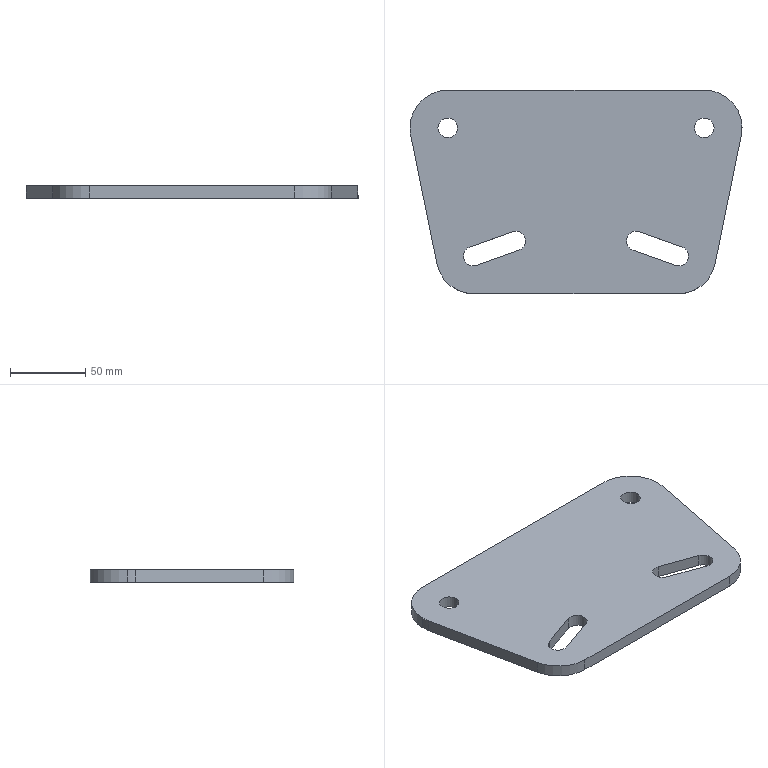Part | SolidWorks | features Extrusion 1 | 1 solid | 25 faces | box 220 x 135 x 8 mm | volume 204896 mm3 | cylinder 15 | plane 10 | commonest cylinder face diameters 13 x10 50 x5
STEP:
#1=CARTESIAN_POINT('',(163.5,-25.,8.));
#2=VERTEX_POINT('',#1);
#3=CARTESIAN_POINT('',(176.5,-25.,8.));
#4=VERTEX_POINT('',#3);
#5=CARTESIAN_POINT('',(170.,-25.,8.));
#6=DIRECTION('',(0.,0.,1.));
#7=DIRECTION('',(1.,0.,0.));
#8=AXIS2_PLACEMENT_3D('',#5,#6,#7);
#9=CIRCLE('',#8,6.5);
#10=EDGE_CURVE('',#2,#4,#9,.T.);
#11=ORIENTED_EDGE('',*,*,#10,.T.);
#12=CARTESIAN_POINT('',(176.5,-25.,0.));
#13=VERTEX_POINT('',#12);
#14=CARTESIAN_POINT('',(176.5,-25.,8.));
#15=DIRECTION('',(0.,0.,-1.));
#16=VECTOR('',#15,1000.);
#17=LINE('',#14,#16);
#18=EDGE_CURVE('',#4,#13,#17,.T.);
#19=ORIENTED_EDGE('',*,*,#18,.T.);
#20=CARTESIAN_POINT('',(163.5,-25.,0.));
#21=VERTEX_POINT('',#20);
#22=CARTESIAN_POINT('',(170.,-25.,0.));
#23=DIRECTION('',(0.,0.,1.));
#24=DIRECTION('',(1.,0.,0.));
#25=AXIS2_PLACEMENT_3D('',#22,#23,#24);
#26=CIRCLE('',#25,6.5);
#27=EDGE_CURVE('',#21,#13,#26,.T.);
#28=ORIENTED_EDGE('',*,*,#27,.F.);
#29=CARTESIAN_POINT('',(163.5,-25.,8.));
#30=DIRECTION('',(0.,0.,-1.));
#31=VECTOR('',#30,1000.);
#32=LINE('',#29,#31);
#33=EDGE_CURVE('',#2,#21,#32,.T.);
#34=ORIENTED_EDGE('',*,*,#33,.F.);
#35=EDGE_LOOP('',(#11,#19,#28,#34));
#36=FACE_OUTER_BOUND('',#35,.T.);
#37=CARTESIAN_POINT('',(170.,-25.,8.));
#38=DIRECTION('',(0.,0.,-1.));
#39=DIRECTION('',(-1.,0.,0.));
#40=AXIS2_PLACEMENT_3D('',#37,#38,#39);
#41=CYLINDRICAL_SURFACE('',#40,6.5);
#42=ADVANCED_FACE('',(#36),#41,.F.);
#43=CARTESIAN_POINT('',(14.814,-103.879,8.));
#44=VERTEX_POINT('',#43);
#45=CARTESIAN_POINT('',(10.5,-110.,8.));
#46=VERTEX_POINT('',#45);
#47=CARTESIAN_POINT('',(17.,-110.,8.));
#48=DIRECTION('',(0.,0.,1.));
#49=DIRECTION('',(1.,0.,0.));
#50=AXIS2_PLACEMENT_3D('',#47,#48,#49);
#51=CIRCLE('',#50,6.5);
#52=EDGE_CURVE('',#44,#46,#51,.T.);
#53=ORIENTED_EDGE('',*,*,#52,.T.);
#54=CARTESIAN_POINT('',(10.5,-110.,0.));
#55=VERTEX_POINT('',#54);
#56=CARTESIAN_POINT('',(10.5,-110.,8.));
#57=DIRECTION('',(0.,0.,-1.));
#58=VECTOR('',#57,1000.);
#59=LINE('',#56,#58);
#60=EDGE_CURVE('',#46,#55,#59,.T.);
#61=ORIENTED_EDGE('',*,*,#60,.T.);
#62=CARTESIAN_POINT('',(14.814,-103.879,0.));
#63=VERTEX_POINT('',#62);
#64=CARTESIAN_POINT('',(17.,-110.,0.));
#65=DIRECTION('',(0.,0.,1.));
#66=DIRECTION('',(1.,0.,0.));
#67=AXIS2_PLACEMENT_3D('',#64,#65,#66);
#68=CIRCLE('',#67,6.5);
#69=EDGE_CURVE('',#63,#55,#68,.T.);
#70=ORIENTED_EDGE('',*,*,#69,.F.);
#71=CARTESIAN_POINT('',(14.814,-103.879,8.));
#72=DIRECTION('',(0.,0.,-1.));
#73=VECTOR('',#72,1000.);
#74=LINE('',#71,#73);
#75=EDGE_CURVE('',#44,#63,#74,.T.);
#76=ORIENTED_EDGE('',*,*,#75,.F.);
#77=EDGE_LOOP('',(#53,#61,#70,#76));
#78=FACE_OUTER_BOUND('',#77,.T.);
#79=CARTESIAN_POINT('',(17.,-110.,8.));
#80=DIRECTION('',(0.,0.,-1.));
#81=DIRECTION('',(-1.,0.,0.));
#82=AXIS2_PLACEMENT_3D('',#79,#80,#81);
#83=CYLINDRICAL_SURFACE('',#82,6.5);
#84=ADVANCED_FACE('',(#78),#83,.F.);
#85=CARTESIAN_POINT('',(127.186,-93.879,8.));
#86=VERTEX_POINT('',#85);
#87=CARTESIAN_POINT('',(118.5,-100.,8.));
#88=VERTEX_POINT('',#87);
#89=CARTESIAN_POINT('',(125.,-100.,8.));
#90=DIRECTION('',(0.,0.,1.));
#91=DIRECTION('',(1.,0.,0.));
#92=AXIS2_PLACEMENT_3D('',#89,#90,#91);
#93=CIRCLE('',#92,6.5);
#94=EDGE_CURVE('',#86,#88,#93,.T.);
#95=ORIENTED_EDGE('',*,*,#94,.T.);
#96=CARTESIAN_POINT('',(118.5,-100.,0.));
#97=VERTEX_POINT('',#96);
#98=CARTESIAN_POINT('',(118.5,-100.,8.));
#99=DIRECTION('',(0.,0.,-1.));
#100=VECTOR('',#99,1000.);
#101=LINE('',#98,#100);
#102=EDGE_CURVE('',#88,#97,#101,.T.);
#103=ORIENTED_EDGE('',*,*,#102,.T.);
#104=CARTESIAN_POINT('',(127.186,-93.879,0.));
#105=VERTEX_POINT('',#104);
#106=CARTESIAN_POINT('',(125.,-100.,0.));
#107=DIRECTION('',(0.,0.,1.));
#108=DIRECTION('',(1.,0.,0.));
#109=AXIS2_PLACEMENT_3D('',#106,#107,#108);
#110=CIRCLE('',#109,6.5);
#111=EDGE_CURVE('',#105,#97,#110,.T.);
#112=ORIENTED_EDGE('',*,*,#111,.F.);
#113=CARTESIAN_POINT('',(127.186,-93.879,8.));
#114=DIRECTION('',(0.,0.,-1.));
#115=VECTOR('',#114,1000.);
#116=LINE('',#113,#115);
#117=EDGE_CURVE('',#86,#105,#116,.T.);
#118=ORIENTED_EDGE('',*,*,#117,.F.);
#119=EDGE_LOOP('',(#95,#103,#112,#118));
#120=FACE_OUTER_BOUND('',#119,.T.);
#121=CARTESIAN_POINT('',(125.,-100.,8.));
#122=DIRECTION('',(0.,0.,-1.));
#123=DIRECTION('',(-1.,0.,0.));
#124=AXIS2_PLACEMENT_3D('',#121,#122,#123);
#125=CYLINDRICAL_SURFACE('',#124,6.5);
#126=ADVANCED_FACE('',(#120),#125,.F.);
#127=CARTESIAN_POINT('',(-6.5,-25.,8.));
#128=VERTEX_POINT('',#127);
#129=CARTESIAN_POINT('',(6.5,-25.,8.));
#130=VERTEX_POINT('',#129);
#131=CARTESIAN_POINT('',(0.,-25.,8.));
#132=DIRECTION('',(0.,0.,1.));
#133=DIRECTION('',(1.,0.,0.));
#134=AXIS2_PLACEMENT_3D('',#131,#132,#133);
#135=CIRCLE('',#134,6.5);
#136=EDGE_CURVE('',#128,#130,#135,.T.);
#137=ORIENTED_EDGE('',*,*,#136,.T.);
#138=CARTESIAN_POINT('',(6.5,-25.,0.));
#139=VERTEX_POINT('',#138);
#140=CARTESIAN_POINT('',(6.5,-25.,8.));
#141=DIRECTION('',(0.,0.,-1.));
#142=VECTOR('',#141,1000.);
#143=LINE('',#140,#142);
#144=EDGE_CURVE('',#130,#139,#143,.T.);
#145=ORIENTED_EDGE('',*,*,#144,.T.);
#146=CARTESIAN_POINT('',(-6.5,-25.,0.));
#147=VERTEX_POINT('',#146);
#148=CARTESIAN_POINT('',(0.,-25.,0.));
#149=DIRECTION('',(0.,0.,1.));
#150=DIRECTION('',(1.,0.,0.));
#151=AXIS2_PLACEMENT_3D('',#148,#149,#150);
#152=CIRCLE('',#151,6.5);
#153=EDGE_CURVE('',#147,#139,#152,.T.);
#154=ORIENTED_EDGE('',*,*,#153,.F.);
#155=CARTESIAN_POINT('',(-6.5,-25.,8.));
#156=DIRECTION('',(0.,0.,-1.));
#157=VECTOR('',#156,1000.);
#158=LINE('',#155,#157);
#159=EDGE_CURVE('',#128,#147,#158,.T.);
#160=ORIENTED_EDGE('',*,*,#159,.F.);
#161=EDGE_LOOP('',(#137,#145,#154,#160));
#162=FACE_OUTER_BOUND('',#161,.T.);
#163=CARTESIAN_POINT('',(0.,-25.,8.));
#164=DIRECTION('',(0.,0.,-1.));
#165=DIRECTION('',(-1.,0.,0.));
#166=AXIS2_PLACEMENT_3D('',#163,#164,#165);
#167=CYLINDRICAL_SURFACE('',#166,6.5);
#168=ADVANCED_FACE('',(#162),#167,.F.);
#169=CARTESIAN_POINT('',(-25.,-25.,8.));
#170=VERTEX_POINT('',#169);
#171=CARTESIAN_POINT('',(-24.498,-29.984,8.));
#172=VERTEX_POINT('',#171);
#173=CARTESIAN_POINT('',(0.,-25.,8.));
#174=DIRECTION('',(0.,0.,1.));
#175=DIRECTION('',(1.,0.,0.));
#176=AXIS2_PLACEMENT_3D('',#173,#174,#175);
#177=CIRCLE('',#176,25.);
#178=EDGE_CURVE('',#170,#172,#177,.T.);
#179=ORIENTED_EDGE('',*,*,#178,.F.);
#180=CARTESIAN_POINT('',(-25.,-25.,0.));
#181=VERTEX_POINT('',#180);
#182=CARTESIAN_POINT('',(-25.,-25.,8.));
#183=DIRECTION('',(0.,0.,-1.));
#184=VECTOR('',#183,1000.);
#185=LINE('',#182,#184);
#186=EDGE_CURVE('',#170,#181,#185,.T.);
#187=ORIENTED_EDGE('',*,*,#186,.T.);
#188=CARTESIAN_POINT('',(-24.498,-29.984,0.));
#189=VERTEX_POINT('',#188);
#190=CARTESIAN_POINT('',(0.,-25.,0.));
#191=DIRECTION('',(0.,0.,1.));
#192=DIRECTION('',(1.,0.,0.));
#193=AXIS2_PLACEMENT_3D('',#190,#191,#192);
#194=CIRCLE('',#193,25.);
#195=EDGE_CURVE('',#181,#189,#194,.T.);
#196=ORIENTED_EDGE('',*,*,#195,.T.);
#197=CARTESIAN_POINT('',(-24.498,-29.984,8.));
#198=DIRECTION('',(0.,0.,-1.));
#199=VECTOR('',#198,1000.);
#200=LINE('',#197,#199);
#201=EDGE_CURVE('',#172,#189,#200,.T.);
#202=ORIENTED_EDGE('',*,*,#201,.F.);
#203=EDGE_LOOP('',(#179,#187,#196,#202));
#204=FACE_OUTER_BOUND('',#203,.T.);
#205=CARTESIAN_POINT('',(0.,-25.,8.));
#206=DIRECTION('',(0.,0.,-1.));
#207=DIRECTION('',(-1.,0.,0.));
#208=AXIS2_PLACEMENT_3D('',#205,#206,#207);
#209=CYLINDRICAL_SURFACE('',#208,25.);
#210=ADVANCED_FACE('',(#204),#209,.T.);
#211=CARTESIAN_POINT('',(47.186,-106.121,8.));
#212=VERTEX_POINT('',#211);
#213=CARTESIAN_POINT('',(42.814,-93.879,8.));
#214=VERTEX_POINT('',#213);
#215=CARTESIAN_POINT('',(45.,-100.,8.));
#216=DIRECTION('',(0.,0.,1.));
#217=DIRECTION('',(1.,0.,0.));
#218=AXIS2_PLACEMENT_3D('',#215,#216,#217);
#219=CIRCLE('',#218,6.5);
#220=EDGE_CURVE('',#212,#214,#219,.T.);
#221=ORIENTED_EDGE('',*,*,#220,.F.);
#222=CARTESIAN_POINT('',(19.186,-116.121,8.));
#223=VERTEX_POINT('',#222);
#224=CARTESIAN_POINT('',(38.951,-109.062,8.));
#225=DIRECTION('',(0.9417,0.3363,0.));
#226=VECTOR('',#225,1000.);
#227=LINE('',#224,#226);
#228=EDGE_CURVE('',#223,#212,#227,.T.);
#229=ORIENTED_EDGE('',*,*,#228,.F.);
#230=CARTESIAN_POINT('',(17.,-110.,8.));
#231=DIRECTION('',(0.,0.,1.));
#232=DIRECTION('',(1.,0.,0.));
#233=AXIS2_PLACEMENT_3D('',#230,#231,#232);
#234=CIRCLE('',#233,6.5);
#235=EDGE_CURVE('',#46,#223,#234,.T.);
#236=ORIENTED_EDGE('',*,*,#235,.F.);
#237=ORIENTED_EDGE('',*,*,#52,.F.);
#238=CARTESIAN_POINT('',(34.579,-96.82,8.));
#239=DIRECTION('',(0.9417,0.3363,0.));
#240=VECTOR('',#239,1000.);
#241=LINE('',#238,#240);
#242=EDGE_CURVE('',#44,#214,#241,.T.);
#243=ORIENTED_EDGE('',*,*,#242,.T.);
#244=EDGE_LOOP('',(#221,#229,#236,#237,#243));
#245=FACE_BOUND('',#244,.T.);
#246=CARTESIAN_POINT('',(150.814,-116.121,8.));
#247=VERTEX_POINT('',#246);
#248=CARTESIAN_POINT('',(155.186,-103.879,8.));
#249=VERTEX_POINT('',#248);
#250=CARTESIAN_POINT('',(153.,-110.,8.));
#251=DIRECTION('',(0.,0.,1.));
#252=DIRECTION('',(1.,0.,0.));
#253=AXIS2_PLACEMENT_3D('',#250,#251,#252);
#254=CIRCLE('',#253,6.5);
#255=EDGE_CURVE('',#247,#249,#254,.T.);
#256=ORIENTED_EDGE('',*,*,#255,.F.);
#257=CARTESIAN_POINT('',(122.814,-106.121,8.));
#258=VERTEX_POINT('',#257);
#259=CARTESIAN_POINT('',(-19.72,-55.216,8.));
#260=DIRECTION('',(0.9417,-0.3363,0.));
#261=VECTOR('',#260,1000.);
#262=LINE('',#259,#261);
#263=EDGE_CURVE('',#258,#247,#262,.T.);
#264=ORIENTED_EDGE('',*,*,#263,.F.);
#265=CARTESIAN_POINT('',(125.,-100.,8.));
#266=DIRECTION('',(0.,0.,1.));
#267=DIRECTION('',(1.,0.,0.));
#268=AXIS2_PLACEMENT_3D('',#265,#266,#267);
#269=CIRCLE('',#268,6.5);
#270=EDGE_CURVE('',#88,#258,#269,.T.);
#271=ORIENTED_EDGE('',*,*,#270,.F.);
#272=ORIENTED_EDGE('',*,*,#94,.F.);
#273=CARTESIAN_POINT('',(-15.348,-42.974,8.));
#274=DIRECTION('',(0.9417,-0.3363,0.));
#275=VECTOR('',#274,1000.);
#276=LINE('',#273,#275);
#277=EDGE_CURVE('',#86,#249,#276,.T.);
#278=ORIENTED_EDGE('',*,*,#277,.T.);
#279=EDGE_LOOP('',(#256,#264,#271,#272,#278));
#280=FACE_BOUND('',#279,.T.);
#281=ORIENTED_EDGE('',*,*,#136,.F.);
#282=CARTESIAN_POINT('',(0.,-25.,8.));
#283=DIRECTION('',(0.,0.,1.));
#284=DIRECTION('',(1.,0.,0.));
#285=AXIS2_PLACEMENT_3D('',#282,#283,#284);
#286=CIRCLE('',#285,6.5);
#287=EDGE_CURVE('',#130,#128,#286,.T.);
#288=ORIENTED_EDGE('',*,*,#287,.F.);
#289=EDGE_LOOP('',(#281,#288));
#290=FACE_BOUND('',#289,.T.);
#291=CARTESIAN_POINT('',(-7.205,-114.984,8.));
#292=VERTEX_POINT('',#291);
#293=CARTESIAN_POINT('',(17.293,-135.,8.));
#294=VERTEX_POINT('',#293);
#295=CARTESIAN_POINT('',(17.293,-110.,8.));
#296=DIRECTION('',(0.,0.,1.));
#297=DIRECTION('',(1.,0.,0.));
#298=AXIS2_PLACEMENT_3D('',#295,#296,#297);
#299=CIRCLE('',#298,25.);
#300=EDGE_CURVE('',#292,#294,#299,.T.);
#301=ORIENTED_EDGE('',*,*,#300,.T.);
#302=CARTESIAN_POINT('',(152.707,-135.,8.));
#303=VERTEX_POINT('',#302);
#304=CARTESIAN_POINT('',(17.293,-135.,8.));
#305=DIRECTION('',(1.,0.,0.));
#306=VECTOR('',#305,1000.);
#307=LINE('',#304,#306);
#308=EDGE_CURVE('',#294,#303,#307,.T.);
#309=ORIENTED_EDGE('',*,*,#308,.T.);
#310=CARTESIAN_POINT('',(177.205,-114.984,8.));
#311=VERTEX_POINT('',#310);
#312=CARTESIAN_POINT('',(152.707,-110.,8.));
#313=DIRECTION('',(0.,0.,-1.));
#314=DIRECTION('',(-1.,0.,0.));
#315=AXIS2_PLACEMENT_3D('',#312,#313,#314);
#316=CIRCLE('',#315,25.);
#317=EDGE_CURVE('',#311,#303,#316,.T.);
#318=ORIENTED_EDGE('',*,*,#317,.F.);
#319=CARTESIAN_POINT('',(194.498,-29.984,8.));
#320=VERTEX_POINT('',#319);
#321=CARTESIAN_POINT('',(194.498,-29.984,8.));
#322=DIRECTION('',(-0.1994,-0.9799,0.));
#323=VECTOR('',#322,1000.);
#324=LINE('',#321,#323);
#325=EDGE_CURVE('',#320,#311,#324,.T.);
#326=ORIENTED_EDGE('',*,*,#325,.F.);
#327=CARTESIAN_POINT('',(170.,0.,8.));
#328=VERTEX_POINT('',#327);
#329=CARTESIAN_POINT('',(170.,-25.,8.));
#330=DIRECTION('',(0.,0.,-1.));
#331=DIRECTION('',(-1.,0.,0.));
#332=AXIS2_PLACEMENT_3D('',#329,#330,#331);
#333=CIRCLE('',#332,25.);
#334=EDGE_CURVE('',#328,#320,#333,.T.);
#335=ORIENTED_EDGE('',*,*,#334,.F.);
#336=CARTESIAN_POINT('',(0.,0.,8.));
#337=VERTEX_POINT('',#336);
#338=CARTESIAN_POINT('',(0.,0.,8.));
#339=DIRECTION('',(1.,0.,0.));
#340=VECTOR('',#339,1000.);
#341=LINE('',#338,#340);
#342=EDGE_CURVE('',#337,#328,#341,.T.);
#343=ORIENTED_EDGE('',*,*,#342,.F.);
#344=CARTESIAN_POINT('',(0.,-25.,8.));
#345=DIRECTION('',(0.,0.,1.));
#346=DIRECTION('',(1.,0.,0.));
#347=AXIS2_PLACEMENT_3D('',#344,#345,#346);
#348=CIRCLE('',#347,25.);
#349=EDGE_CURVE('',#337,#170,#348,.T.);
#350=ORIENTED_EDGE('',*,*,#349,.T.);
#351=ORIENTED_EDGE('',*,*,#178,.T.);
#352=CARTESIAN_POINT('',(-24.498,-29.984,8.));
#353=DIRECTION('',(0.1994,-0.9799,0.));
#354=VECTOR('',#353,1000.);
#355=LINE('',#352,#354);
#356=EDGE_CURVE('',#172,#292,#355,.T.);
#357=ORIENTED_EDGE('',*,*,#356,.T.);
#358=EDGE_LOOP('',(#301,#309,#318,#326,#335,#343,#350,#351,#357));
#359=FACE_OUTER_BOUND('',#358,.T.);
#360=ORIENTED_EDGE('',*,*,#10,.F.);
#361=CARTESIAN_POINT('',(170.,-25.,8.));
#362=DIRECTION('',(0.,0.,1.));
#363=DIRECTION('',(1.,0.,0.));
#364=AXIS2_PLACEMENT_3D('',#361,#362,#363);
#365=CIRCLE('',#364,6.5);
#366=EDGE_CURVE('',#4,#2,#365,.T.);
#367=ORIENTED_EDGE('',*,*,#366,.F.);
#368=EDGE_LOOP('',(#360,#367));
#369=FACE_BOUND('',#368,.T.);
#370=CARTESIAN_POINT('',(17.293,-110.,8.));
#371=DIRECTION('',(0.,0.,1.));
#372=DIRECTION('',(1.,0.,0.));
#373=AXIS2_PLACEMENT_3D('',#370,#371,#372);
#374=PLANE('',#373);
#375=ADVANCED_FACE('',(#245,#280,#290,#359,#369),#374,.T.);
#376=CARTESIAN_POINT('',(122.814,-106.121,0.));
#377=VERTEX_POINT('',#376);
#378=CARTESIAN_POINT('',(150.814,-116.121,0.));
#379=VERTEX_POINT('',#378);
#380=CARTESIAN_POINT('',(-19.72,-55.216,0.));
#381=DIRECTION('',(0.9417,-0.3363,0.));
#382=VECTOR('',#381,1000.);
#383=LINE('',#380,#382);
#384=EDGE_CURVE('',#377,#379,#383,.T.);
#385=ORIENTED_EDGE('',*,*,#384,.T.);
#386=CARTESIAN_POINT('',(155.186,-103.879,0.));
#387=VERTEX_POINT('',#386);
#388=CARTESIAN_POINT('',(153.,-110.,0.));
#389=DIRECTION('',(0.,0.,1.));
#390=DIRECTION('',(1.,0.,0.));
#391=AXIS2_PLACEMENT_3D('',#388,#389,#390);
#392=CIRCLE('',#391,6.5);
#393=EDGE_CURVE('',#379,#387,#392,.T.);
#394=ORIENTED_EDGE('',*,*,#393,.T.);
#395=CARTESIAN_POINT('',(-15.348,-42.974,0.));
#396=DIRECTION('',(0.9417,-0.3363,0.));
#397=VECTOR('',#396,1000.);
#398=LINE('',#395,#397);
#399=EDGE_CURVE('',#105,#387,#398,.T.);
#400=ORIENTED_EDGE('',*,*,#399,.F.);
#401=ORIENTED_EDGE('',*,*,#111,.T.);
#402=CARTESIAN_POINT('',(125.,-100.,0.));
#403=DIRECTION('',(0.,0.,1.));
#404=DIRECTION('',(1.,0.,0.));
#405=AXIS2_PLACEMENT_3D('',#402,#403,#404);
#406=CIRCLE('',#405,6.5);
#407=EDGE_CURVE('',#97,#377,#406,.T.);
#408=ORIENTED_EDGE('',*,*,#407,.T.);
#409=EDGE_LOOP('',(#385,#394,#400,#401,#408));
#410=FACE_BOUND('',#409,.T.);
#411=CARTESIAN_POINT('',(-7.205,-114.984,0.));
#412=VERTEX_POINT('',#411);
#413=CARTESIAN_POINT('',(17.293,-135.,0.));
#414=VERTEX_POINT('',#413);
#415=CARTESIAN_POINT('',(17.293,-110.,0.));
#416=DIRECTION('',(0.,0.,1.));
#417=DIRECTION('',(1.,0.,0.));
#418=AXIS2_PLACEMENT_3D('',#415,#416,#417);
#419=CIRCLE('',#418,25.);
#420=EDGE_CURVE('',#412,#414,#419,.T.);
#421=ORIENTED_EDGE('',*,*,#420,.F.);
#422=CARTESIAN_POINT('',(-24.498,-29.984,0.));
#423=DIRECTION('',(0.1994,-0.9799,0.));
#424=VECTOR('',#423,1000.);
#425=LINE('',#422,#424);
#426=EDGE_CURVE('',#189,#412,#425,.T.);
#427=ORIENTED_EDGE('',*,*,#426,.F.);
#428=ORIENTED_EDGE('',*,*,#195,.F.);
#429=CARTESIAN_POINT('',(0.,0.,0.));
#430=VERTEX_POINT('',#429);
#431=CARTESIAN_POINT('',(0.,-25.,0.));
#432=DIRECTION('',(0.,0.,1.));
#433=DIRECTION('',(1.,0.,0.));
#434=AXIS2_PLACEMENT_3D('',#431,#432,#433);
#435=CIRCLE('',#434,25.);
#436=EDGE_CURVE('',#430,#181,#435,.T.);
#437=ORIENTED_EDGE('',*,*,#436,.F.);
#438=CARTESIAN_POINT('',(170.,0.,0.));
#439=VERTEX_POINT('',#438);
#440=CARTESIAN_POINT('',(0.,0.,0.));
#441=DIRECTION('',(1.,0.,0.));
#442=VECTOR('',#441,1000.);
#443=LINE('',#440,#442);
#444=EDGE_CURVE('',#430,#439,#443,.T.);
#445=ORIENTED_EDGE('',*,*,#444,.T.);
#446=CARTESIAN_POINT('',(194.498,-29.984,0.));
#447=VERTEX_POINT('',#446);
#448=CARTESIAN_POINT('',(170.,-25.,0.));
#449=DIRECTION('',(0.,0.,-1.));
#450=DIRECTION('',(-1.,0.,0.));
#451=AXIS2_PLACEMENT_3D('',#448,#449,#450);
#452=CIRCLE('',#451,25.);
#453=EDGE_CURVE('',#439,#447,#452,.T.);
#454=ORIENTED_EDGE('',*,*,#453,.T.);
#455=CARTESIAN_POINT('',(177.205,-114.984,0.));
#456=VERTEX_POINT('',#455);
#457=CARTESIAN_POINT('',(194.498,-29.984,0.));
#458=DIRECTION('',(-0.1994,-0.9799,0.));
#459=VECTOR('',#458,1000.);
#460=LINE('',#457,#459);
#461=EDGE_CURVE('',#447,#456,#460,.T.);
#462=ORIENTED_EDGE('',*,*,#461,.T.);
#463=CARTESIAN_POINT('',(152.707,-135.,0.));
#464=VERTEX_POINT('',#463);
#465=CARTESIAN_POINT('',(152.707,-110.,0.));
#466=DIRECTION('',(0.,0.,-1.));
#467=DIRECTION('',(-1.,0.,0.));
#468=AXIS2_PLACEMENT_3D('',#465,#466,#467);
#469=CIRCLE('',#468,25.);
#470=EDGE_CURVE('',#456,#464,#469,.T.);
#471=ORIENTED_EDGE('',*,*,#470,.T.);
#472=CARTESIAN_POINT('',(17.293,-135.,0.));
#473=DIRECTION('',(1.,0.,0.));
#474=VECTOR('',#473,1000.);
#475=LINE('',#472,#474);
#476=EDGE_CURVE('',#414,#464,#475,.T.);
#477=ORIENTED_EDGE('',*,*,#476,.F.);
#478=EDGE_LOOP('',(#421,#427,#428,#437,#445,#454,#462,#471,#477));
#479=FACE_OUTER_BOUND('',#478,.T.);
#480=ORIENTED_EDGE('',*,*,#153,.T.);
#481=CARTESIAN_POINT('',(0.,-25.,0.));
#482=DIRECTION('',(0.,0.,1.));
#483=DIRECTION('',(1.,0.,0.));
#484=AXIS2_PLACEMENT_3D('',#481,#482,#483);
#485=CIRCLE('',#484,6.5);
#486=EDGE_CURVE('',#139,#147,#485,.T.);
#487=ORIENTED_EDGE('',*,*,#486,.T.);
#488=EDGE_LOOP('',(#480,#487));
#489=FACE_BOUND('',#488,.T.);
#490=CARTESIAN_POINT('',(19.186,-116.121,0.));
#491=VERTEX_POINT('',#490);
#492=CARTESIAN_POINT('',(47.186,-106.121,0.));
#493=VERTEX_POINT('',#492);
#494=CARTESIAN_POINT('',(38.951,-109.062,0.));
#495=DIRECTION('',(0.9417,0.3363,0.));
#496=VECTOR('',#495,1000.);
#497=LINE('',#494,#496);
#498=EDGE_CURVE('',#491,#493,#497,.T.);
#499=ORIENTED_EDGE('',*,*,#498,.T.);
#500=CARTESIAN_POINT('',(42.814,-93.879,0.));
#501=VERTEX_POINT('',#500);
#502=CARTESIAN_POINT('',(45.,-100.,0.));
#503=DIRECTION('',(0.,0.,1.));
#504=DIRECTION('',(1.,0.,0.));
#505=AXIS2_PLACEMENT_3D('',#502,#503,#504);
#506=CIRCLE('',#505,6.5);
#507=EDGE_CURVE('',#493,#501,#506,.T.);
#508=ORIENTED_EDGE('',*,*,#507,.T.);
#509=CARTESIAN_POINT('',(34.579,-96.82,0.));
#510=DIRECTION('',(0.9417,0.3363,0.));
#511=VECTOR('',#510,1000.);
#512=LINE('',#509,#511);
#513=EDGE_CURVE('',#63,#501,#512,.T.);
#514=ORIENTED_EDGE('',*,*,#513,.F.);
#515=ORIENTED_EDGE('',*,*,#69,.T.);
#516=CARTESIAN_POINT('',(17.,-110.,0.));
#517=DIRECTION('',(0.,0.,1.));
#518=DIRECTION('',(1.,0.,0.));
#519=AXIS2_PLACEMENT_3D('',#516,#517,#518);
#520=CIRCLE('',#519,6.5);
#521=EDGE_CURVE('',#55,#491,#520,.T.);
#522=ORIENTED_EDGE('',*,*,#521,.T.);
#523=EDGE_LOOP('',(#499,#508,#514,#515,#522));
#524=FACE_BOUND('',#523,.T.);
#525=ORIENTED_EDGE('',*,*,#27,.T.);
#526=CARTESIAN_POINT('',(170.,-25.,0.));
#527=DIRECTION('',(0.,0.,1.));
#528=DIRECTION('',(1.,0.,0.));
#529=AXIS2_PLACEMENT_3D('',#526,#527,#528);
#530=CIRCLE('',#529,6.5);
#531=EDGE_CURVE('',#13,#21,#530,.T.);
#532=ORIENTED_EDGE('',*,*,#531,.T.);
#533=EDGE_LOOP('',(#525,#532));
#534=FACE_BOUND('',#533,.T.);
#535=CARTESIAN_POINT('',(17.293,-110.,0.));
#536=DIRECTION('',(0.,0.,1.));
#537=DIRECTION('',(1.,0.,0.));
#538=AXIS2_PLACEMENT_3D('',#535,#536,#537);
#539=PLANE('',#538);
#540=ADVANCED_FACE('',(#410,#479,#489,#524,#534),#539,.F.);
#541=ORIENTED_EDGE('',*,*,#420,.T.);
#542=CARTESIAN_POINT('',(17.293,-135.,8.));
#543=DIRECTION('',(0.,0.,-1.));
#544=VECTOR('',#543,1000.);
#545=LINE('',#542,#544);
#546=EDGE_CURVE('',#294,#414,#545,.T.);
#547=ORIENTED_EDGE('',*,*,#546,.F.);
#548=ORIENTED_EDGE('',*,*,#300,.F.);
#549=CARTESIAN_POINT('',(-7.205,-114.984,8.));
#550=DIRECTION('',(0.,0.,-1.));
#551=VECTOR('',#550,1000.);
#552=LINE('',#549,#551);
#553=EDGE_CURVE('',#292,#412,#552,.T.);
#554=ORIENTED_EDGE('',*,*,#553,.T.);
#555=EDGE_LOOP('',(#541,#547,#548,#554));
#556=FACE_OUTER_BOUND('',#555,.T.);
#557=CARTESIAN_POINT('',(17.293,-110.,8.));
#558=DIRECTION('',(0.,0.,-1.));
#559=DIRECTION('',(-1.,0.,0.));
#560=AXIS2_PLACEMENT_3D('',#557,#558,#559);
#561=CYLINDRICAL_SURFACE('',#560,25.);
#562=ADVANCED_FACE('',(#556),#561,.T.);
#563=ORIENTED_EDGE('',*,*,#476,.T.);
#564=CARTESIAN_POINT('',(152.707,-135.,8.));
#565=DIRECTION('',(0.,0.,-1.));
#566=VECTOR('',#565,1000.);
#567=LINE('',#564,#566);
#568=EDGE_CURVE('',#303,#464,#567,.T.);
#569=ORIENTED_EDGE('',*,*,#568,.F.);
#570=ORIENTED_EDGE('',*,*,#308,.F.);
#571=ORIENTED_EDGE('',*,*,#546,.T.);
#572=EDGE_LOOP('',(#563,#569,#570,#571));
#573=FACE_OUTER_BOUND('',#572,.T.);
#574=CARTESIAN_POINT('',(17.293,-135.,8.));
#575=DIRECTION('',(0.,1.,0.));
#576=DIRECTION('',(0.,0.,1.));
#577=AXIS2_PLACEMENT_3D('',#574,#575,#576);
#578=PLANE('',#577);
#579=ADVANCED_FACE('',(#573),#578,.F.);
#580=ORIENTED_EDGE('',*,*,#470,.F.);
#581=CARTESIAN_POINT('',(177.205,-114.984,8.));
#582=DIRECTION('',(0.,0.,-1.));
#583=VECTOR('',#582,1000.);
#584=LINE('',#581,#583);
#585=EDGE_CURVE('',#311,#456,#584,.T.);
#586=ORIENTED_EDGE('',*,*,#585,.F.);
#587=ORIENTED_EDGE('',*,*,#317,.T.);
#588=ORIENTED_EDGE('',*,*,#568,.T.);
#589=EDGE_LOOP('',(#580,#586,#587,#588));
#590=FACE_OUTER_BOUND('',#589,.T.);
#591=CARTESIAN_POINT('',(152.707,-110.,8.));
#592=DIRECTION('',(0.,0.,-1.));
#593=DIRECTION('',(-1.,0.,0.));
#594=AXIS2_PLACEMENT_3D('',#591,#592,#593);
#595=CYLINDRICAL_SURFACE('',#594,25.);
#596=ADVANCED_FACE('',(#590),#595,.T.);
#597=ORIENTED_EDGE('',*,*,#461,.F.);
#598=CARTESIAN_POINT('',(194.498,-29.984,8.));
#599=DIRECTION('',(0.,0.,-1.));
#600=VECTOR('',#599,1000.);
#601=LINE('',#598,#600);
#602=EDGE_CURVE('',#320,#447,#601,.T.);
#603=ORIENTED_EDGE('',*,*,#602,.F.);
#604=ORIENTED_EDGE('',*,*,#325,.T.);
#605=ORIENTED_EDGE('',*,*,#585,.T.);
#606=EDGE_LOOP('',(#597,#603,#604,#605));
#607=FACE_OUTER_BOUND('',#606,.T.);
#608=CARTESIAN_POINT('',(194.498,-29.984,8.));
#609=DIRECTION('',(0.9799,-0.1994,0.));
#610=DIRECTION('',(0.1994,0.9799,0.));
#611=AXIS2_PLACEMENT_3D('',#608,#609,#610);
#612=PLANE('',#611);
#613=ADVANCED_FACE('',(#607),#612,.T.);
#614=ORIENTED_EDGE('',*,*,#453,.F.);
#615=CARTESIAN_POINT('',(170.,0.,8.));
#616=DIRECTION('',(0.,0.,-1.));
#617=VECTOR('',#616,1000.);
#618=LINE('',#615,#617);
#619=EDGE_CURVE('',#328,#439,#618,.T.);
#620=ORIENTED_EDGE('',*,*,#619,.F.);
#621=ORIENTED_EDGE('',*,*,#334,.T.);
#622=ORIENTED_EDGE('',*,*,#602,.T.);
#623=EDGE_LOOP('',(#614,#620,#621,#622));
#624=FACE_OUTER_BOUND('',#623,.T.);
#625=CARTESIAN_POINT('',(170.,-25.,8.));
#626=DIRECTION('',(0.,0.,-1.));
#627=DIRECTION('',(-1.,0.,0.));
#628=AXIS2_PLACEMENT_3D('',#625,#626,#627);
#629=CYLINDRICAL_SURFACE('',#628,25.);
#630=ADVANCED_FACE('',(#624),#629,.T.);
#631=ORIENTED_EDGE('',*,*,#444,.F.);
#632=CARTESIAN_POINT('',(0.,0.,8.));
#633=DIRECTION('',(0.,0.,-1.));
#634=VECTOR('',#633,1000.);
#635=LINE('',#632,#634);
#636=EDGE_CURVE('',#337,#430,#635,.T.);
#637=ORIENTED_EDGE('',*,*,#636,.F.);
#638=ORIENTED_EDGE('',*,*,#342,.T.);
#639=ORIENTED_EDGE('',*,*,#619,.T.);
#640=EDGE_LOOP('',(#631,#637,#638,#639));
#641=FACE_OUTER_BOUND('',#640,.T.);
#642=CARTESIAN_POINT('',(0.,0.,8.));
#643=DIRECTION('',(0.,1.,0.));
#644=DIRECTION('',(-1.,0.,0.));
#645=AXIS2_PLACEMENT_3D('',#642,#643,#644);
#646=PLANE('',#645);
#647=ADVANCED_FACE('',(#641),#646,.T.);
#648=ORIENTED_EDGE('',*,*,#186,.F.);
#649=ORIENTED_EDGE('',*,*,#349,.F.);
#650=ORIENTED_EDGE('',*,*,#636,.T.);
#651=ORIENTED_EDGE('',*,*,#436,.T.);
#652=EDGE_LOOP('',(#648,#649,#650,#651));
#653=FACE_OUTER_BOUND('',#652,.T.);
#654=CARTESIAN_POINT('',(0.,-25.,8.));
#655=DIRECTION('',(0.,0.,-1.));
#656=DIRECTION('',(-1.,0.,0.));
#657=AXIS2_PLACEMENT_3D('',#654,#655,#656);
#658=CYLINDRICAL_SURFACE('',#657,25.);
#659=ADVANCED_FACE('',(#653),#658,.T.);
#660=ORIENTED_EDGE('',*,*,#426,.T.);
#661=ORIENTED_EDGE('',*,*,#553,.F.);
#662=ORIENTED_EDGE('',*,*,#356,.F.);
#663=ORIENTED_EDGE('',*,*,#201,.T.);
#664=EDGE_LOOP('',(#660,#661,#662,#663));
#665=FACE_OUTER_BOUND('',#664,.T.);
#666=CARTESIAN_POINT('',(-24.498,-29.984,8.));
#667=DIRECTION('',(0.9799,0.1994,0.));
#668=DIRECTION('',(-0.1994,0.9799,0.));
#669=AXIS2_PLACEMENT_3D('',#666,#667,#668);
#670=PLANE('',#669);
#671=ADVANCED_FACE('',(#665),#670,.F.);
#672=ORIENTED_EDGE('',*,*,#144,.F.);
#673=ORIENTED_EDGE('',*,*,#287,.T.);
#674=ORIENTED_EDGE('',*,*,#159,.T.);
#675=ORIENTED_EDGE('',*,*,#486,.F.);
#676=EDGE_LOOP('',(#672,#673,#674,#675));
#677=FACE_OUTER_BOUND('',#676,.T.);
#678=CARTESIAN_POINT('',(0.,-25.,8.));
#679=DIRECTION('',(0.,0.,-1.));
#680=DIRECTION('',(-1.,0.,0.));
#681=AXIS2_PLACEMENT_3D('',#678,#679,#680);
#682=CYLINDRICAL_SURFACE('',#681,6.5);
#683=ADVANCED_FACE('',(#677),#682,.F.);
#684=ORIENTED_EDGE('',*,*,#384,.F.);
#685=CARTESIAN_POINT('',(122.814,-106.121,8.));
#686=DIRECTION('',(0.,0.,-1.));
#687=VECTOR('',#686,1000.);
#688=LINE('',#685,#687);
#689=EDGE_CURVE('',#258,#377,#688,.T.);
#690=ORIENTED_EDGE('',*,*,#689,.F.);
#691=ORIENTED_EDGE('',*,*,#263,.T.);
#692=CARTESIAN_POINT('',(150.814,-116.121,8.));
#693=DIRECTION('',(0.,0.,-1.));
#694=VECTOR('',#693,1000.);
#695=LINE('',#692,#694);
#696=EDGE_CURVE('',#247,#379,#695,.T.);
#697=ORIENTED_EDGE('',*,*,#696,.T.);
#698=EDGE_LOOP('',(#684,#690,#691,#697));
#699=FACE_OUTER_BOUND('',#698,.T.);
#700=CARTESIAN_POINT('',(-19.72,-55.216,8.));
#701=DIRECTION('',(0.3363,0.9417,0.));
#702=DIRECTION('',(-0.9417,0.3363,0.));
#703=AXIS2_PLACEMENT_3D('',#700,#701,#702);
#704=PLANE('',#703);
#705=ADVANCED_FACE('',(#699),#704,.T.);
#706=ORIENTED_EDGE('',*,*,#393,.F.);
#707=ORIENTED_EDGE('',*,*,#696,.F.);
#708=ORIENTED_EDGE('',*,*,#255,.T.);
#709=CARTESIAN_POINT('',(155.186,-103.879,8.));
#710=DIRECTION('',(0.,0.,-1.));
#711=VECTOR('',#710,1000.);
#712=LINE('',#709,#711);
#713=EDGE_CURVE('',#249,#387,#712,.T.);
#714=ORIENTED_EDGE('',*,*,#713,.T.);
#715=EDGE_LOOP('',(#706,#707,#708,#714));
#716=FACE_OUTER_BOUND('',#715,.T.);
#717=CARTESIAN_POINT('',(153.,-110.,8.));
#718=DIRECTION('',(0.,0.,-1.));
#719=DIRECTION('',(-1.,0.,0.));
#720=AXIS2_PLACEMENT_3D('',#717,#718,#719);
#721=CYLINDRICAL_SURFACE('',#720,6.5);
#722=ADVANCED_FACE('',(#716),#721,.F.);
#723=ORIENTED_EDGE('',*,*,#399,.T.);
#724=ORIENTED_EDGE('',*,*,#713,.F.);
#725=ORIENTED_EDGE('',*,*,#277,.F.);
#726=ORIENTED_EDGE('',*,*,#117,.T.);
#727=EDGE_LOOP('',(#723,#724,#725,#726));
#728=FACE_OUTER_BOUND('',#727,.T.);
#729=CARTESIAN_POINT('',(-15.348,-42.974,8.));
#730=DIRECTION('',(0.3363,0.9417,0.));
#731=DIRECTION('',(-0.9417,0.3363,0.));
#732=AXIS2_PLACEMENT_3D('',#729,#730,#731);
#733=PLANE('',#732);
#734=ADVANCED_FACE('',(#728),#733,.F.);
#735=ORIENTED_EDGE('',*,*,#102,.F.);
#736=ORIENTED_EDGE('',*,*,#270,.T.);
#737=ORIENTED_EDGE('',*,*,#689,.T.);
#738=ORIENTED_EDGE('',*,*,#407,.F.);
#739=EDGE_LOOP('',(#735,#736,#737,#738));
#740=FACE_OUTER_BOUND('',#739,.T.);
#741=CARTESIAN_POINT('',(125.,-100.,8.));
#742=DIRECTION('',(0.,0.,-1.));
#743=DIRECTION('',(-1.,0.,0.));
#744=AXIS2_PLACEMENT_3D('',#741,#742,#743);
#745=CYLINDRICAL_SURFACE('',#744,6.5);
#746=ADVANCED_FACE('',(#740),#745,.F.);
#747=ORIENTED_EDGE('',*,*,#498,.F.);
#748=CARTESIAN_POINT('',(19.186,-116.121,8.));
#749=DIRECTION('',(0.,0.,-1.));
#750=VECTOR('',#749,1000.);
#751=LINE('',#748,#750);
#752=EDGE_CURVE('',#223,#491,#751,.T.);
#753=ORIENTED_EDGE('',*,*,#752,.F.);
#754=ORIENTED_EDGE('',*,*,#228,.T.);
#755=CARTESIAN_POINT('',(47.186,-106.121,8.));
#756=DIRECTION('',(0.,0.,-1.));
#757=VECTOR('',#756,1000.);
#758=LINE('',#755,#757);
#759=EDGE_CURVE('',#212,#493,#758,.T.);
#760=ORIENTED_EDGE('',*,*,#759,.T.);
#761=EDGE_LOOP('',(#747,#753,#754,#760));
#762=FACE_OUTER_BOUND('',#761,.T.);
#763=CARTESIAN_POINT('',(38.951,-109.062,8.));
#764=DIRECTION('',(-0.3363,0.9417,0.));
#765=DIRECTION('',(-0.9417,-0.3363,0.));
#766=AXIS2_PLACEMENT_3D('',#763,#764,#765);
#767=PLANE('',#766);
#768=ADVANCED_FACE('',(#762),#767,.T.);
#769=ORIENTED_EDGE('',*,*,#507,.F.);
#770=ORIENTED_EDGE('',*,*,#759,.F.);
#771=ORIENTED_EDGE('',*,*,#220,.T.);
#772=CARTESIAN_POINT('',(42.814,-93.879,8.));
#773=DIRECTION('',(0.,0.,-1.));
#774=VECTOR('',#773,1000.);
#775=LINE('',#772,#774);
#776=EDGE_CURVE('',#214,#501,#775,.T.);
#777=ORIENTED_EDGE('',*,*,#776,.T.);
#778=EDGE_LOOP('',(#769,#770,#771,#777));
#779=FACE_OUTER_BOUND('',#778,.T.);
#780=CARTESIAN_POINT('',(45.,-100.,8.));
#781=DIRECTION('',(0.,0.,-1.));
#782=DIRECTION('',(-1.,0.,0.));
#783=AXIS2_PLACEMENT_3D('',#780,#781,#782);
#784=CYLINDRICAL_SURFACE('',#783,6.5);
#785=ADVANCED_FACE('',(#779),#784,.F.);
#786=ORIENTED_EDGE('',*,*,#513,.T.);
#787=ORIENTED_EDGE('',*,*,#776,.F.);
#788=ORIENTED_EDGE('',*,*,#242,.F.);
#789=ORIENTED_EDGE('',*,*,#75,.T.);
#790=EDGE_LOOP('',(#786,#787,#788,#789));
#791=FACE_OUTER_BOUND('',#790,.T.);
#792=CARTESIAN_POINT('',(34.579,-96.82,8.));
#793=DIRECTION('',(-0.3363,0.9417,0.));
#794=DIRECTION('',(-0.9417,-0.3363,0.));
#795=AXIS2_PLACEMENT_3D('',#792,#793,#794);
#796=PLANE('',#795);
#797=ADVANCED_FACE('',(#791),#796,.F.);
#798=ORIENTED_EDGE('',*,*,#60,.F.);
#799=ORIENTED_EDGE('',*,*,#235,.T.);
#800=ORIENTED_EDGE('',*,*,#752,.T.);
#801=ORIENTED_EDGE('',*,*,#521,.F.);
#802=EDGE_LOOP('',(#798,#799,#800,#801));
#803=FACE_OUTER_BOUND('',#802,.T.);
#804=CARTESIAN_POINT('',(17.,-110.,8.));
#805=DIRECTION('',(0.,0.,-1.));
#806=DIRECTION('',(-1.,0.,0.));
#807=AXIS2_PLACEMENT_3D('',#804,#805,#806);
#808=CYLINDRICAL_SURFACE('',#807,6.5);
#809=ADVANCED_FACE('',(#803),#808,.F.);
#810=ORIENTED_EDGE('',*,*,#18,.F.);
#811=ORIENTED_EDGE('',*,*,#366,.T.);
#812=ORIENTED_EDGE('',*,*,#33,.T.);
#813=ORIENTED_EDGE('',*,*,#531,.F.);
#814=EDGE_LOOP('',(#810,#811,#812,#813));
#815=FACE_OUTER_BOUND('',#814,.T.);
#816=CARTESIAN_POINT('',(170.,-25.,8.));
#817=DIRECTION('',(0.,0.,-1.));
#818=DIRECTION('',(-1.,0.,0.));
#819=AXIS2_PLACEMENT_3D('',#816,#817,#818);
#820=CYLINDRICAL_SURFACE('',#819,6.5);
#821=ADVANCED_FACE('',(#815),#820,.F.);
#822=CLOSED_SHELL('',(#42,#84,#126,#168,#210,#375,#540,#562,#579,#596,#613,#630,#647,#659,#671,#683,#705,#722,#734,#746,#768,#785,#797,#809,#821));
#823=MANIFOLD_SOLID_BREP('',#822);
#824=CARTESIAN_POINT('',(0.,0.,0.));
#825=DIRECTION('',(0.,0.,1.));
#826=DIRECTION('',(1.,0.,0.));
#827=AXIS2_PLACEMENT_3D('',#824,#825,#826);
#828=(LENGTH_UNIT()NAMED_UNIT(*)SI_UNIT(.MILLI.,.METRE.));
#829=UNCERTAINTY_MEASURE_WITH_UNIT(LENGTH_MEASURE(0.00001),#828,'','');
#830=(NAMED_UNIT(*)PLANE_ANGLE_UNIT()SI_UNIT($,.RADIAN.));
#831=(NAMED_UNIT(*)SI_UNIT($,.STERADIAN.)SOLID_ANGLE_UNIT());
#832=(GEOMETRIC_REPRESENTATION_CONTEXT(3)GLOBAL_UNCERTAINTY_ASSIGNED_CONTEXT((#829))GLOBAL_UNIT_ASSIGNED_CONTEXT((#828,#830,#831))REPRESENTATION_CONTEXT('',''));
#833=ADVANCED_BREP_SHAPE_REPRESENTATION('',(#823,#827),#832);